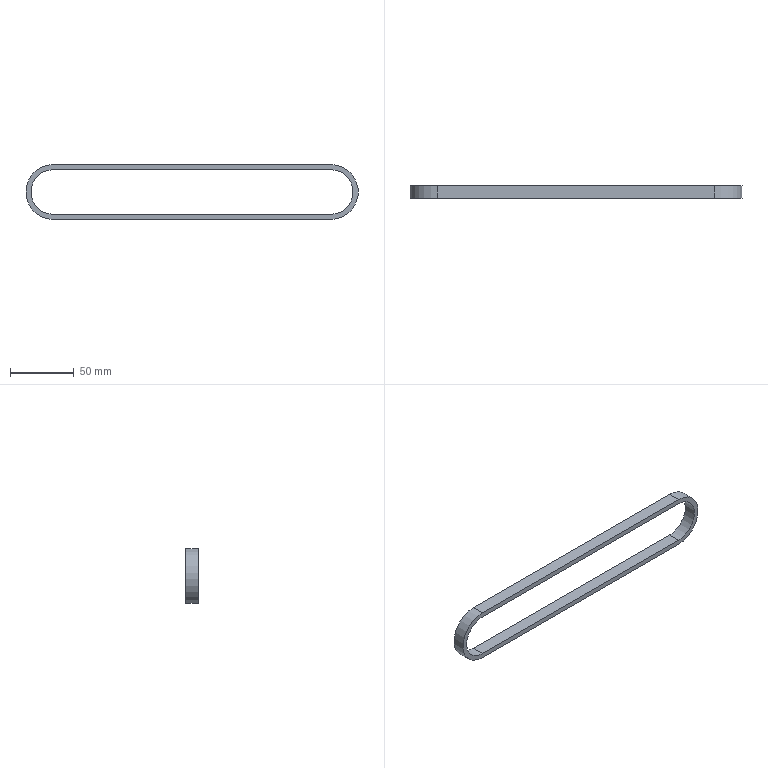Part | STEP file | 10000020550swp000-1 | 1 solid | 10 faces | box 260.44 x 10 x 43.01 mm | volume 22297 mm3 | plane 6 | cylinder 4 | commonest cylinder face diameters 35.01 x2 43.01 x2
STEP:
#1=CARTESIAN_POINT('',(0.,10.,-21.505));
#2=VERTEX_POINT('',#1);
#3=CARTESIAN_POINT('',(0.,10.,21.505));
#4=VERTEX_POINT('',#3);
#5=CARTESIAN_POINT('',(0.,10.,0.));
#6=DIRECTION('',(0.,1.,0.));
#7=DIRECTION('',(1.,0.,0.));
#8=AXIS2_PLACEMENT_3D('',#5,#6,#7);
#9=CIRCLE('',#8,21.505);
#10=EDGE_CURVE('',#2,#4,#9,.T.);
#11=ORIENTED_EDGE('',*,*,#10,.T.);
#12=CARTESIAN_POINT('',(217.43,10.,21.505));
#13=VERTEX_POINT('',#12);
#14=CARTESIAN_POINT('',(0.,10.,21.505));
#15=DIRECTION('',(1.,0.,0.));
#16=VECTOR('',#15,1000.);
#17=LINE('',#14,#16);
#18=EDGE_CURVE('',#4,#13,#17,.T.);
#19=ORIENTED_EDGE('',*,*,#18,.T.);
#20=CARTESIAN_POINT('',(217.43,10.,-21.505));
#21=VERTEX_POINT('',#20);
#22=CARTESIAN_POINT('',(217.43,10.,0.));
#23=DIRECTION('',(0.,1.,0.));
#24=DIRECTION('',(1.,0.,0.));
#25=AXIS2_PLACEMENT_3D('',#22,#23,#24);
#26=CIRCLE('',#25,21.505);
#27=EDGE_CURVE('',#13,#21,#26,.T.);
#28=ORIENTED_EDGE('',*,*,#27,.T.);
#29=CARTESIAN_POINT('',(0.,10.,-21.505));
#30=DIRECTION('',(1.,0.,0.));
#31=VECTOR('',#30,1000.);
#32=LINE('',#29,#31);
#33=EDGE_CURVE('',#2,#21,#32,.T.);
#34=ORIENTED_EDGE('',*,*,#33,.F.);
#35=EDGE_LOOP('',(#11,#19,#28,#34));
#36=FACE_OUTER_BOUND('',#35,.T.);
#37=CARTESIAN_POINT('',(0.,10.,17.505));
#38=VERTEX_POINT('',#37);
#39=CARTESIAN_POINT('',(217.43,10.,17.505));
#40=VERTEX_POINT('',#39);
#41=CARTESIAN_POINT('',(0.,10.,17.505));
#42=DIRECTION('',(1.,0.,0.));
#43=VECTOR('',#42,1000.);
#44=LINE('',#41,#43);
#45=EDGE_CURVE('',#38,#40,#44,.T.);
#46=ORIENTED_EDGE('',*,*,#45,.F.);
#47=CARTESIAN_POINT('',(0.,10.,-17.505));
#48=VERTEX_POINT('',#47);
#49=CARTESIAN_POINT('',(0.,10.,0.));
#50=DIRECTION('',(0.,1.,0.));
#51=DIRECTION('',(0.,0.,1.));
#52=AXIS2_PLACEMENT_3D('',#49,#50,#51);
#53=CIRCLE('',#52,17.505);
#54=EDGE_CURVE('',#48,#38,#53,.T.);
#55=ORIENTED_EDGE('',*,*,#54,.F.);
#56=CARTESIAN_POINT('',(217.43,10.,-17.505));
#57=VERTEX_POINT('',#56);
#58=CARTESIAN_POINT('',(0.,10.,-17.505));
#59=DIRECTION('',(1.,0.,0.));
#60=VECTOR('',#59,1000.);
#61=LINE('',#58,#60);
#62=EDGE_CURVE('',#48,#57,#61,.T.);
#63=ORIENTED_EDGE('',*,*,#62,.T.);
#64=CARTESIAN_POINT('',(217.43,10.,0.));
#65=DIRECTION('',(0.,1.,0.));
#66=DIRECTION('',(0.,0.,1.));
#67=AXIS2_PLACEMENT_3D('',#64,#65,#66);
#68=CIRCLE('',#67,17.505);
#69=EDGE_CURVE('',#40,#57,#68,.T.);
#70=ORIENTED_EDGE('',*,*,#69,.F.);
#71=EDGE_LOOP('',(#46,#55,#63,#70));
#72=FACE_BOUND('',#71,.T.);
#73=CARTESIAN_POINT('',(0.,10.,0.));
#74=DIRECTION('',(0.,1.,0.));
#75=DIRECTION('',(0.,0.,1.));
#76=AXIS2_PLACEMENT_3D('',#73,#74,#75);
#77=PLANE('',#76);
#78=ADVANCED_FACE('',(#36,#72),#77,.T.);
#79=CARTESIAN_POINT('',(0.,0.,-21.505));
#80=VERTEX_POINT('',#79);
#81=CARTESIAN_POINT('',(0.,0.,21.505));
#82=VERTEX_POINT('',#81);
#83=CARTESIAN_POINT('',(0.,0.,0.));
#84=DIRECTION('',(0.,1.,0.));
#85=DIRECTION('',(1.,0.,0.));
#86=AXIS2_PLACEMENT_3D('',#83,#84,#85);
#87=CIRCLE('',#86,21.505);
#88=EDGE_CURVE('',#80,#82,#87,.T.);
#89=ORIENTED_EDGE('',*,*,#88,.F.);
#90=CARTESIAN_POINT('',(217.43,0.,-21.505));
#91=VERTEX_POINT('',#90);
#92=CARTESIAN_POINT('',(0.,0.,-21.505));
#93=DIRECTION('',(1.,0.,0.));
#94=VECTOR('',#93,1000.);
#95=LINE('',#92,#94);
#96=EDGE_CURVE('',#80,#91,#95,.T.);
#97=ORIENTED_EDGE('',*,*,#96,.T.);
#98=CARTESIAN_POINT('',(217.43,0.,21.505));
#99=VERTEX_POINT('',#98);
#100=CARTESIAN_POINT('',(217.43,0.,0.));
#101=DIRECTION('',(0.,1.,0.));
#102=DIRECTION('',(1.,0.,0.));
#103=AXIS2_PLACEMENT_3D('',#100,#101,#102);
#104=CIRCLE('',#103,21.505);
#105=EDGE_CURVE('',#99,#91,#104,.T.);
#106=ORIENTED_EDGE('',*,*,#105,.F.);
#107=CARTESIAN_POINT('',(0.,0.,21.505));
#108=DIRECTION('',(1.,0.,0.));
#109=VECTOR('',#108,1000.);
#110=LINE('',#107,#109);
#111=EDGE_CURVE('',#82,#99,#110,.T.);
#112=ORIENTED_EDGE('',*,*,#111,.F.);
#113=EDGE_LOOP('',(#89,#97,#106,#112));
#114=FACE_OUTER_BOUND('',#113,.T.);
#115=CARTESIAN_POINT('',(0.,0.,-17.505));
#116=VERTEX_POINT('',#115);
#117=CARTESIAN_POINT('',(0.,0.,17.505));
#118=VERTEX_POINT('',#117);
#119=CARTESIAN_POINT('',(0.,0.,0.));
#120=DIRECTION('',(0.,1.,0.));
#121=DIRECTION('',(0.,0.,1.));
#122=AXIS2_PLACEMENT_3D('',#119,#120,#121);
#123=CIRCLE('',#122,17.505);
#124=EDGE_CURVE('',#116,#118,#123,.T.);
#125=ORIENTED_EDGE('',*,*,#124,.T.);
#126=CARTESIAN_POINT('',(217.43,0.,17.505));
#127=VERTEX_POINT('',#126);
#128=CARTESIAN_POINT('',(0.,0.,17.505));
#129=DIRECTION('',(1.,0.,0.));
#130=VECTOR('',#129,1000.);
#131=LINE('',#128,#130);
#132=EDGE_CURVE('',#118,#127,#131,.T.);
#133=ORIENTED_EDGE('',*,*,#132,.T.);
#134=CARTESIAN_POINT('',(217.43,0.,-17.505));
#135=VERTEX_POINT('',#134);
#136=CARTESIAN_POINT('',(217.43,0.,0.));
#137=DIRECTION('',(0.,1.,0.));
#138=DIRECTION('',(0.,0.,1.));
#139=AXIS2_PLACEMENT_3D('',#136,#137,#138);
#140=CIRCLE('',#139,17.505);
#141=EDGE_CURVE('',#127,#135,#140,.T.);
#142=ORIENTED_EDGE('',*,*,#141,.T.);
#143=CARTESIAN_POINT('',(0.,0.,-17.505));
#144=DIRECTION('',(1.,0.,0.));
#145=VECTOR('',#144,1000.);
#146=LINE('',#143,#145);
#147=EDGE_CURVE('',#116,#135,#146,.T.);
#148=ORIENTED_EDGE('',*,*,#147,.F.);
#149=EDGE_LOOP('',(#125,#133,#142,#148));
#150=FACE_BOUND('',#149,.T.);
#151=CARTESIAN_POINT('',(0.,0.,0.));
#152=DIRECTION('',(0.,1.,0.));
#153=DIRECTION('',(0.,0.,1.));
#154=AXIS2_PLACEMENT_3D('',#151,#152,#153);
#155=PLANE('',#154);
#156=ADVANCED_FACE('',(#114,#150),#155,.F.);
#157=ORIENTED_EDGE('',*,*,#88,.T.);
#158=CARTESIAN_POINT('',(0.,10.,21.505));
#159=DIRECTION('',(0.,-1.,0.));
#160=VECTOR('',#159,1000.);
#161=LINE('',#158,#160);
#162=EDGE_CURVE('',#4,#82,#161,.T.);
#163=ORIENTED_EDGE('',*,*,#162,.F.);
#164=ORIENTED_EDGE('',*,*,#10,.F.);
#165=CARTESIAN_POINT('',(0.,10.,-21.505));
#166=DIRECTION('',(0.,-1.,0.));
#167=VECTOR('',#166,1000.);
#168=LINE('',#165,#167);
#169=EDGE_CURVE('',#2,#80,#168,.T.);
#170=ORIENTED_EDGE('',*,*,#169,.T.);
#171=EDGE_LOOP('',(#157,#163,#164,#170));
#172=FACE_OUTER_BOUND('',#171,.T.);
#173=CARTESIAN_POINT('',(0.,10.,0.));
#174=DIRECTION('',(0.,-1.,0.));
#175=DIRECTION('',(0.,0.,-1.));
#176=AXIS2_PLACEMENT_3D('',#173,#174,#175);
#177=CYLINDRICAL_SURFACE('',#176,21.505);
#178=ADVANCED_FACE('',(#172),#177,.T.);
#179=ORIENTED_EDGE('',*,*,#111,.T.);
#180=CARTESIAN_POINT('',(217.43,10.,21.505));
#181=DIRECTION('',(0.,-1.,0.));
#182=VECTOR('',#181,1000.);
#183=LINE('',#180,#182);
#184=EDGE_CURVE('',#13,#99,#183,.T.);
#185=ORIENTED_EDGE('',*,*,#184,.F.);
#186=ORIENTED_EDGE('',*,*,#18,.F.);
#187=ORIENTED_EDGE('',*,*,#162,.T.);
#188=EDGE_LOOP('',(#179,#185,#186,#187));
#189=FACE_OUTER_BOUND('',#188,.T.);
#190=CARTESIAN_POINT('',(0.,10.,21.505));
#191=DIRECTION('',(0.,0.,-1.));
#192=DIRECTION('',(-1.,0.,0.));
#193=AXIS2_PLACEMENT_3D('',#190,#191,#192);
#194=PLANE('',#193);
#195=ADVANCED_FACE('',(#189),#194,.F.);
#196=ORIENTED_EDGE('',*,*,#105,.T.);
#197=CARTESIAN_POINT('',(217.43,10.,-21.505));
#198=DIRECTION('',(0.,-1.,0.));
#199=VECTOR('',#198,1000.);
#200=LINE('',#197,#199);
#201=EDGE_CURVE('',#21,#91,#200,.T.);
#202=ORIENTED_EDGE('',*,*,#201,.F.);
#203=ORIENTED_EDGE('',*,*,#27,.F.);
#204=ORIENTED_EDGE('',*,*,#184,.T.);
#205=EDGE_LOOP('',(#196,#202,#203,#204));
#206=FACE_OUTER_BOUND('',#205,.T.);
#207=CARTESIAN_POINT('',(217.43,10.,0.));
#208=DIRECTION('',(0.,-1.,0.));
#209=DIRECTION('',(0.,0.,-1.));
#210=AXIS2_PLACEMENT_3D('',#207,#208,#209);
#211=CYLINDRICAL_SURFACE('',#210,21.505);
#212=ADVANCED_FACE('',(#206),#211,.T.);
#213=ORIENTED_EDGE('',*,*,#96,.F.);
#214=ORIENTED_EDGE('',*,*,#169,.F.);
#215=ORIENTED_EDGE('',*,*,#33,.T.);
#216=ORIENTED_EDGE('',*,*,#201,.T.);
#217=EDGE_LOOP('',(#213,#214,#215,#216));
#218=FACE_OUTER_BOUND('',#217,.T.);
#219=CARTESIAN_POINT('',(0.,10.,-21.505));
#220=DIRECTION('',(0.,0.,-1.));
#221=DIRECTION('',(-1.,0.,0.));
#222=AXIS2_PLACEMENT_3D('',#219,#220,#221);
#223=PLANE('',#222);
#224=ADVANCED_FACE('',(#218),#223,.T.);
#225=ORIENTED_EDGE('',*,*,#124,.F.);
#226=CARTESIAN_POINT('',(0.,10.,-17.505));
#227=DIRECTION('',(0.,-1.,0.));
#228=VECTOR('',#227,1000.);
#229=LINE('',#226,#228);
#230=EDGE_CURVE('',#48,#116,#229,.T.);
#231=ORIENTED_EDGE('',*,*,#230,.F.);
#232=ORIENTED_EDGE('',*,*,#54,.T.);
#233=CARTESIAN_POINT('',(0.,10.,17.505));
#234=DIRECTION('',(0.,-1.,0.));
#235=VECTOR('',#234,1000.);
#236=LINE('',#233,#235);
#237=EDGE_CURVE('',#38,#118,#236,.T.);
#238=ORIENTED_EDGE('',*,*,#237,.T.);
#239=EDGE_LOOP('',(#225,#231,#232,#238));
#240=FACE_OUTER_BOUND('',#239,.T.);
#241=CARTESIAN_POINT('',(0.,10.,0.));
#242=DIRECTION('',(0.,-1.,0.));
#243=DIRECTION('',(0.,0.,-1.));
#244=AXIS2_PLACEMENT_3D('',#241,#242,#243);
#245=CYLINDRICAL_SURFACE('',#244,17.505);
#246=ADVANCED_FACE('',(#240),#245,.F.);
#247=ORIENTED_EDGE('',*,*,#132,.F.);
#248=ORIENTED_EDGE('',*,*,#237,.F.);
#249=ORIENTED_EDGE('',*,*,#45,.T.);
#250=CARTESIAN_POINT('',(217.43,10.,17.505));
#251=DIRECTION('',(0.,-1.,0.));
#252=VECTOR('',#251,1000.);
#253=LINE('',#250,#252);
#254=EDGE_CURVE('',#40,#127,#253,.T.);
#255=ORIENTED_EDGE('',*,*,#254,.T.);
#256=EDGE_LOOP('',(#247,#248,#249,#255));
#257=FACE_OUTER_BOUND('',#256,.T.);
#258=CARTESIAN_POINT('',(0.,10.,17.505));
#259=DIRECTION('',(0.,0.,-1.));
#260=DIRECTION('',(-1.,0.,0.));
#261=AXIS2_PLACEMENT_3D('',#258,#259,#260);
#262=PLANE('',#261);
#263=ADVANCED_FACE('',(#257),#262,.T.);
#264=ORIENTED_EDGE('',*,*,#141,.F.);
#265=ORIENTED_EDGE('',*,*,#254,.F.);
#266=ORIENTED_EDGE('',*,*,#69,.T.);
#267=CARTESIAN_POINT('',(217.43,10.,-17.505));
#268=DIRECTION('',(0.,-1.,0.));
#269=VECTOR('',#268,1000.);
#270=LINE('',#267,#269);
#271=EDGE_CURVE('',#57,#135,#270,.T.);
#272=ORIENTED_EDGE('',*,*,#271,.T.);
#273=EDGE_LOOP('',(#264,#265,#266,#272));
#274=FACE_OUTER_BOUND('',#273,.T.);
#275=CARTESIAN_POINT('',(217.43,10.,0.));
#276=DIRECTION('',(0.,-1.,0.));
#277=DIRECTION('',(0.,0.,-1.));
#278=AXIS2_PLACEMENT_3D('',#275,#276,#277);
#279=CYLINDRICAL_SURFACE('',#278,17.505);
#280=ADVANCED_FACE('',(#274),#279,.F.);
#281=ORIENTED_EDGE('',*,*,#147,.T.);
#282=ORIENTED_EDGE('',*,*,#271,.F.);
#283=ORIENTED_EDGE('',*,*,#62,.F.);
#284=ORIENTED_EDGE('',*,*,#230,.T.);
#285=EDGE_LOOP('',(#281,#282,#283,#284));
#286=FACE_OUTER_BOUND('',#285,.T.);
#287=CARTESIAN_POINT('',(0.,10.,-17.505));
#288=DIRECTION('',(0.,0.,-1.));
#289=DIRECTION('',(-1.,0.,0.));
#290=AXIS2_PLACEMENT_3D('',#287,#288,#289);
#291=PLANE('',#290);
#292=ADVANCED_FACE('',(#286),#291,.F.);
#293=CLOSED_SHELL('',(#78,#156,#178,#195,#212,#224,#246,#263,#280,#292));
#294=MANIFOLD_SOLID_BREP('',#293);
#295=CARTESIAN_POINT('',(0.,0.,0.));
#296=DIRECTION('',(0.,0.,1.));
#297=DIRECTION('',(1.,0.,0.));
#298=AXIS2_PLACEMENT_3D('',#295,#296,#297);
#299=(LENGTH_UNIT()NAMED_UNIT(*)SI_UNIT(.MILLI.,.METRE.));
#300=UNCERTAINTY_MEASURE_WITH_UNIT(LENGTH_MEASURE(0.00001),#299,'','');
#301=(NAMED_UNIT(*)PLANE_ANGLE_UNIT()SI_UNIT($,.RADIAN.));
#302=(NAMED_UNIT(*)SI_UNIT($,.STERADIAN.)SOLID_ANGLE_UNIT());
#303=(GEOMETRIC_REPRESENTATION_CONTEXT(3)GLOBAL_UNCERTAINTY_ASSIGNED_CONTEXT((#300))GLOBAL_UNIT_ASSIGNED_CONTEXT((#299,#301,#302))REPRESENTATION_CONTEXT('',''));
#304=ADVANCED_BREP_SHAPE_REPRESENTATION('',(#294,#298),#303);